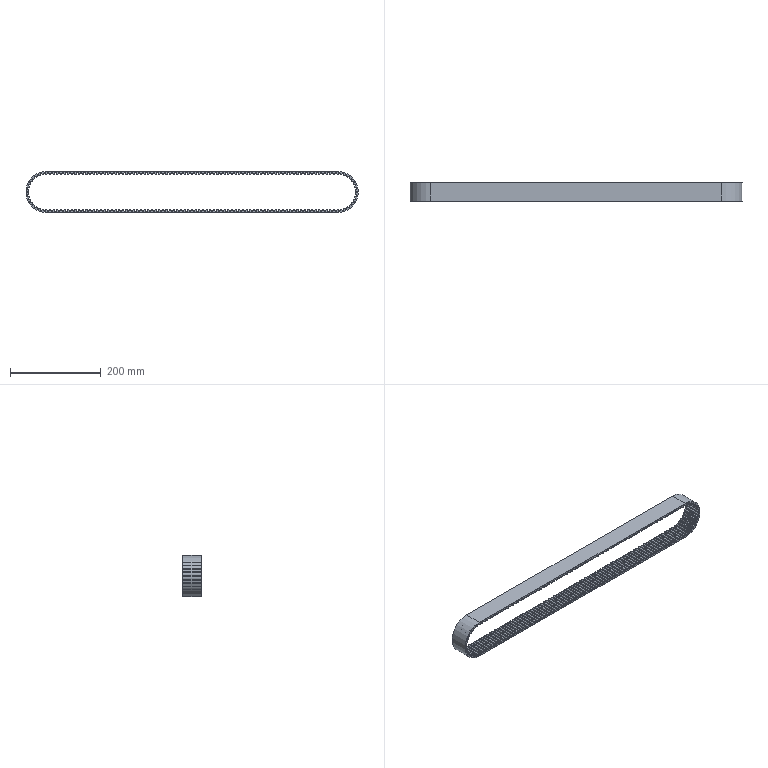Part | SolidWorks | features BaseBody 1 | 1 solid | 1620 faces | box 730.448 x 40 x 90.448 mm | volume 277178 mm3 | plane 814 | cylinder 806 | commonest cylinder face diameters 1.5 x402 4.92 x402 90.448 x2